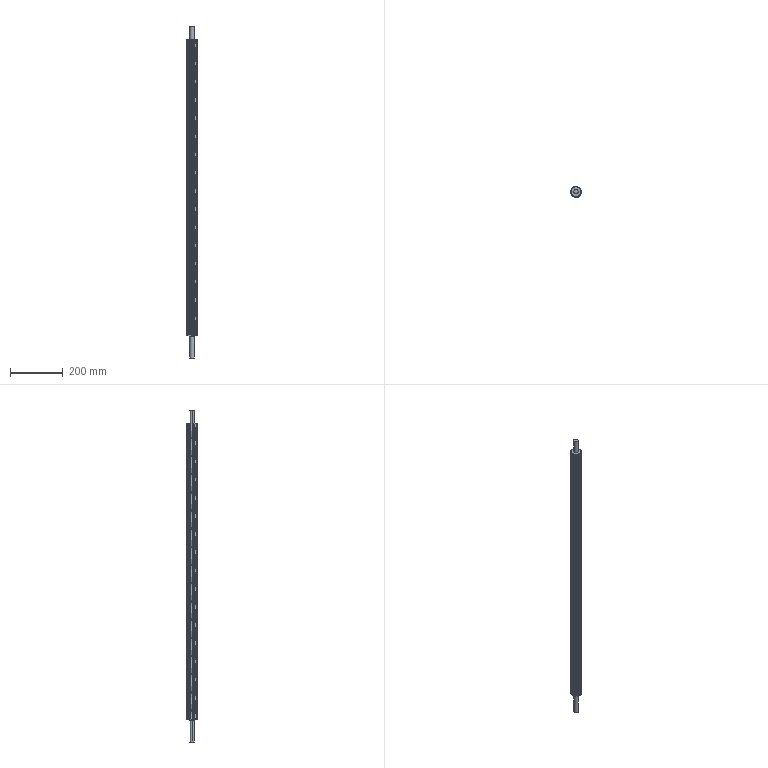Part | SolidWorks | features BaseBody 1 | 1 solid | 591 faces | box 40 x 40 x 1255 mm | volume 1332392 mm3 | cylinder 565 | spline 20 | plane 4 | torus 2 | commonest cylinder face diameters 40 x561 17 x4